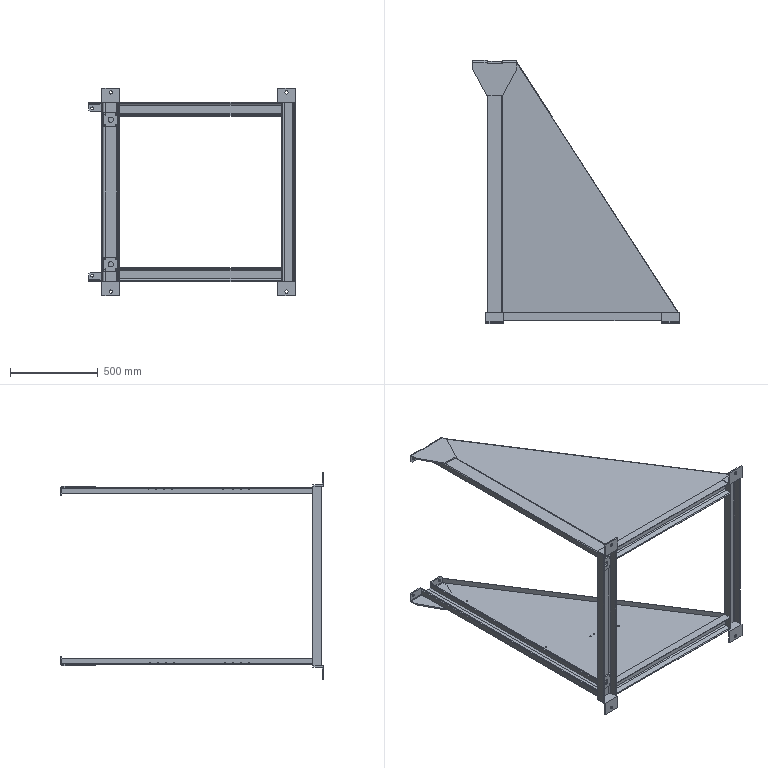Part | SolidWorks | 16 solids | 320 faces | box 1175 x 1495 x 1182 mm | volume 13027521 mm3 | plane 168 | cylinder 136 | cone 16 | commonest cylinder face diameters 5 x36 6.8 x32 7 x12 8 x10 10 x8 15 x8